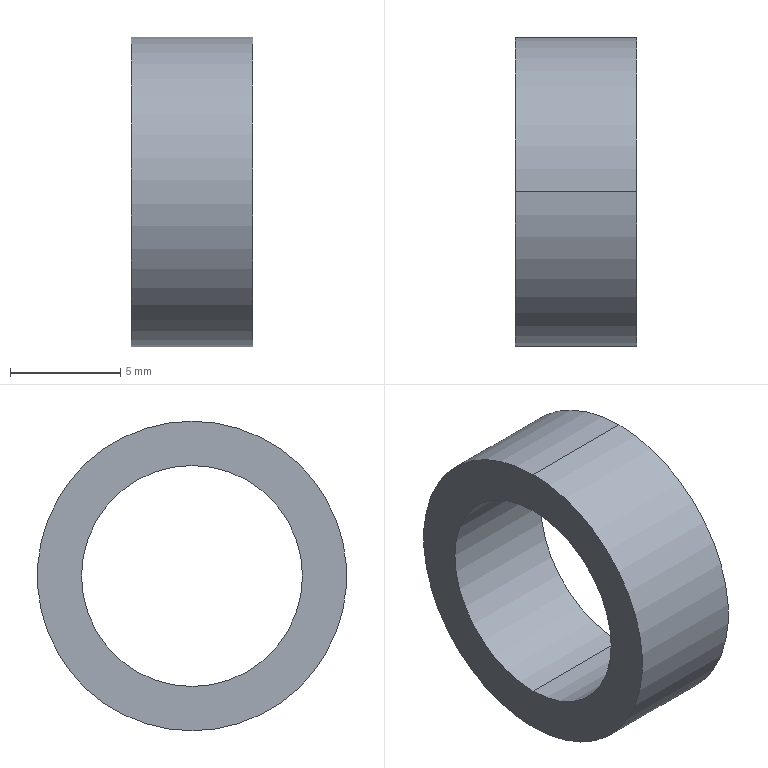Part | SolidWorks | features BaseBody 1 | 1 solid | 6 faces | box 5.5 x 14 x 14 mm | volume 414.69 mm3 | cylinder 4 | plane 2 | commonest cylinder face diameters 10 x2 14 x2
STEP:
#1=CARTESIAN_POINT('',(26.5,0.,7.));
#2=VERTEX_POINT('',#1);
#3=CARTESIAN_POINT('',(26.5,0.,-7.));
#4=VERTEX_POINT('',#3);
#5=CARTESIAN_POINT('',(26.5,0.,0.));
#6=DIRECTION('',(-1.,0.,0.));
#7=DIRECTION('',(0.,0.,1.));
#8=AXIS2_PLACEMENT_3D('',#5,#6,#7);
#9=CIRCLE('',#8,7.);
#10=EDGE_CURVE('',#2,#4,#9,.T.);
#11=ORIENTED_EDGE('',*,*,#10,.T.);
#12=CARTESIAN_POINT('',(21.,0.,-7.));
#13=VERTEX_POINT('',#12);
#14=CARTESIAN_POINT('',(21.,0.,-7.));
#15=DIRECTION('',(-1.,0.,0.));
#16=VECTOR('',#15,1000.);
#17=LINE('',#14,#16);
#18=EDGE_CURVE('',#4,#13,#17,.T.);
#19=ORIENTED_EDGE('',*,*,#18,.T.);
#20=CARTESIAN_POINT('',(21.,0.,7.));
#21=VERTEX_POINT('',#20);
#22=CARTESIAN_POINT('',(21.,0.,0.));
#23=DIRECTION('',(1.,0.,0.));
#24=DIRECTION('',(0.,0.,1.));
#25=AXIS2_PLACEMENT_3D('',#22,#23,#24);
#26=CIRCLE('',#25,7.);
#27=EDGE_CURVE('',#13,#21,#26,.T.);
#28=ORIENTED_EDGE('',*,*,#27,.T.);
#29=CARTESIAN_POINT('',(21.,0.,7.));
#30=DIRECTION('',(-1.,0.,0.));
#31=VECTOR('',#30,1000.);
#32=LINE('',#29,#31);
#33=EDGE_CURVE('',#2,#21,#32,.T.);
#34=ORIENTED_EDGE('',*,*,#33,.F.);
#35=EDGE_LOOP('',(#11,#19,#28,#34));
#36=FACE_OUTER_BOUND('',#35,.T.);
#37=CARTESIAN_POINT('',(21.,0.,0.));
#38=DIRECTION('',(-1.,0.,0.));
#39=DIRECTION('',(0.,0.,1.));
#40=AXIS2_PLACEMENT_3D('',#37,#38,#39);
#41=CYLINDRICAL_SURFACE('',#40,7.);
#42=ADVANCED_FACE('',(#36),#41,.T.);
#43=CARTESIAN_POINT('',(26.5,0.,-5.));
#44=VERTEX_POINT('',#43);
#45=CARTESIAN_POINT('',(26.5,0.,5.));
#46=VERTEX_POINT('',#45);
#47=CARTESIAN_POINT('',(26.5,0.,0.));
#48=DIRECTION('',(-1.,0.,0.));
#49=DIRECTION('',(0.,0.,1.));
#50=AXIS2_PLACEMENT_3D('',#47,#48,#49);
#51=CIRCLE('',#50,5.);
#52=EDGE_CURVE('',#44,#46,#51,.T.);
#53=ORIENTED_EDGE('',*,*,#52,.F.);
#54=CARTESIAN_POINT('',(21.,0.,-5.));
#55=VERTEX_POINT('',#54);
#56=CARTESIAN_POINT('',(21.,0.,-5.));
#57=DIRECTION('',(-1.,0.,0.));
#58=VECTOR('',#57,1000.);
#59=LINE('',#56,#58);
#60=EDGE_CURVE('',#44,#55,#59,.T.);
#61=ORIENTED_EDGE('',*,*,#60,.T.);
#62=CARTESIAN_POINT('',(21.,0.,5.));
#63=VERTEX_POINT('',#62);
#64=CARTESIAN_POINT('',(21.,0.,0.));
#65=DIRECTION('',(-1.,0.,0.));
#66=DIRECTION('',(0.,0.,1.));
#67=AXIS2_PLACEMENT_3D('',#64,#65,#66);
#68=CIRCLE('',#67,5.);
#69=EDGE_CURVE('',#55,#63,#68,.T.);
#70=ORIENTED_EDGE('',*,*,#69,.T.);
#71=CARTESIAN_POINT('',(21.,0.,5.));
#72=DIRECTION('',(-1.,0.,0.));
#73=VECTOR('',#72,1000.);
#74=LINE('',#71,#73);
#75=EDGE_CURVE('',#46,#63,#74,.T.);
#76=ORIENTED_EDGE('',*,*,#75,.F.);
#77=EDGE_LOOP('',(#53,#61,#70,#76));
#78=FACE_OUTER_BOUND('',#77,.T.);
#79=CARTESIAN_POINT('',(21.,0.,0.));
#80=DIRECTION('',(-1.,0.,0.));
#81=DIRECTION('',(0.,0.,1.));
#82=AXIS2_PLACEMENT_3D('',#79,#80,#81);
#83=CYLINDRICAL_SURFACE('',#82,5.);
#84=ADVANCED_FACE('',(#78),#83,.F.);
#85=ORIENTED_EDGE('',*,*,#18,.F.);
#86=CARTESIAN_POINT('',(26.5,0.,0.));
#87=DIRECTION('',(-1.,0.,0.));
#88=DIRECTION('',(0.,0.,1.));
#89=AXIS2_PLACEMENT_3D('',#86,#87,#88);
#90=CIRCLE('',#89,7.);
#91=EDGE_CURVE('',#4,#2,#90,.T.);
#92=ORIENTED_EDGE('',*,*,#91,.T.);
#93=ORIENTED_EDGE('',*,*,#33,.T.);
#94=CARTESIAN_POINT('',(21.,0.,0.));
#95=DIRECTION('',(1.,0.,0.));
#96=DIRECTION('',(0.,0.,1.));
#97=AXIS2_PLACEMENT_3D('',#94,#95,#96);
#98=CIRCLE('',#97,7.);
#99=EDGE_CURVE('',#21,#13,#98,.T.);
#100=ORIENTED_EDGE('',*,*,#99,.T.);
#101=EDGE_LOOP('',(#85,#92,#93,#100));
#102=FACE_OUTER_BOUND('',#101,.T.);
#103=CARTESIAN_POINT('',(21.,0.,0.));
#104=DIRECTION('',(-1.,0.,0.));
#105=DIRECTION('',(0.,0.,1.));
#106=AXIS2_PLACEMENT_3D('',#103,#104,#105);
#107=CYLINDRICAL_SURFACE('',#106,7.);
#108=ADVANCED_FACE('',(#102),#107,.T.);
#109=CARTESIAN_POINT('',(26.5,0.,0.));
#110=DIRECTION('',(-1.,0.,0.));
#111=DIRECTION('',(0.,0.,1.));
#112=AXIS2_PLACEMENT_3D('',#109,#110,#111);
#113=CIRCLE('',#112,5.);
#114=EDGE_CURVE('',#46,#44,#113,.T.);
#115=ORIENTED_EDGE('',*,*,#114,.T.);
#116=ORIENTED_EDGE('',*,*,#52,.T.);
#117=EDGE_LOOP('',(#115,#116));
#118=FACE_BOUND('',#117,.T.);
#119=ORIENTED_EDGE('',*,*,#10,.F.);
#120=ORIENTED_EDGE('',*,*,#91,.F.);
#121=EDGE_LOOP('',(#119,#120));
#122=FACE_OUTER_BOUND('',#121,.T.);
#123=CARTESIAN_POINT('',(26.5,0.,0.));
#124=DIRECTION('',(1.,0.,0.));
#125=DIRECTION('',(0.,0.,-1.));
#126=AXIS2_PLACEMENT_3D('',#123,#124,#125);
#127=PLANE('',#126);
#128=ADVANCED_FACE('',(#118,#122),#127,.T.);
#129=CARTESIAN_POINT('',(21.,0.,0.));
#130=DIRECTION('',(-1.,0.,0.));
#131=DIRECTION('',(0.,0.,1.));
#132=AXIS2_PLACEMENT_3D('',#129,#130,#131);
#133=CIRCLE('',#132,5.);
#134=EDGE_CURVE('',#63,#55,#133,.T.);
#135=ORIENTED_EDGE('',*,*,#134,.F.);
#136=ORIENTED_EDGE('',*,*,#69,.F.);
#137=EDGE_LOOP('',(#135,#136));
#138=FACE_BOUND('',#137,.T.);
#139=ORIENTED_EDGE('',*,*,#99,.F.);
#140=ORIENTED_EDGE('',*,*,#27,.F.);
#141=EDGE_LOOP('',(#139,#140));
#142=FACE_OUTER_BOUND('',#141,.T.);
#143=CARTESIAN_POINT('',(21.,0.,0.));
#144=DIRECTION('',(1.,0.,0.));
#145=DIRECTION('',(0.,0.,-1.));
#146=AXIS2_PLACEMENT_3D('',#143,#144,#145);
#147=PLANE('',#146);
#148=ADVANCED_FACE('',(#138,#142),#147,.F.);
#149=ORIENTED_EDGE('',*,*,#60,.F.);
#150=ORIENTED_EDGE('',*,*,#114,.F.);
#151=ORIENTED_EDGE('',*,*,#75,.T.);
#152=ORIENTED_EDGE('',*,*,#134,.T.);
#153=EDGE_LOOP('',(#149,#150,#151,#152));
#154=FACE_OUTER_BOUND('',#153,.T.);
#155=CARTESIAN_POINT('',(21.,0.,0.));
#156=DIRECTION('',(-1.,0.,0.));
#157=DIRECTION('',(0.,0.,1.));
#158=AXIS2_PLACEMENT_3D('',#155,#156,#157);
#159=CYLINDRICAL_SURFACE('',#158,5.);
#160=ADVANCED_FACE('',(#154),#159,.F.);
#161=CLOSED_SHELL('',(#42,#84,#108,#128,#148,#160));
#162=MANIFOLD_SOLID_BREP('',#161);
#163=CARTESIAN_POINT('',(0.,0.,0.));
#164=DIRECTION('',(0.,0.,1.));
#165=DIRECTION('',(1.,0.,0.));
#166=AXIS2_PLACEMENT_3D('',#163,#164,#165);
#167=(LENGTH_UNIT()NAMED_UNIT(*)SI_UNIT(.MILLI.,.METRE.));
#168=UNCERTAINTY_MEASURE_WITH_UNIT(LENGTH_MEASURE(0.00001),#167,'','');
#169=(NAMED_UNIT(*)PLANE_ANGLE_UNIT()SI_UNIT($,.RADIAN.));
#170=(NAMED_UNIT(*)SI_UNIT($,.STERADIAN.)SOLID_ANGLE_UNIT());
#171=(GEOMETRIC_REPRESENTATION_CONTEXT(3)GLOBAL_UNCERTAINTY_ASSIGNED_CONTEXT((#168))GLOBAL_UNIT_ASSIGNED_CONTEXT((#167,#169,#170))REPRESENTATION_CONTEXT('',''));
#172=ADVANCED_BREP_SHAPE_REPRESENTATION('',(#162,#166),#171);